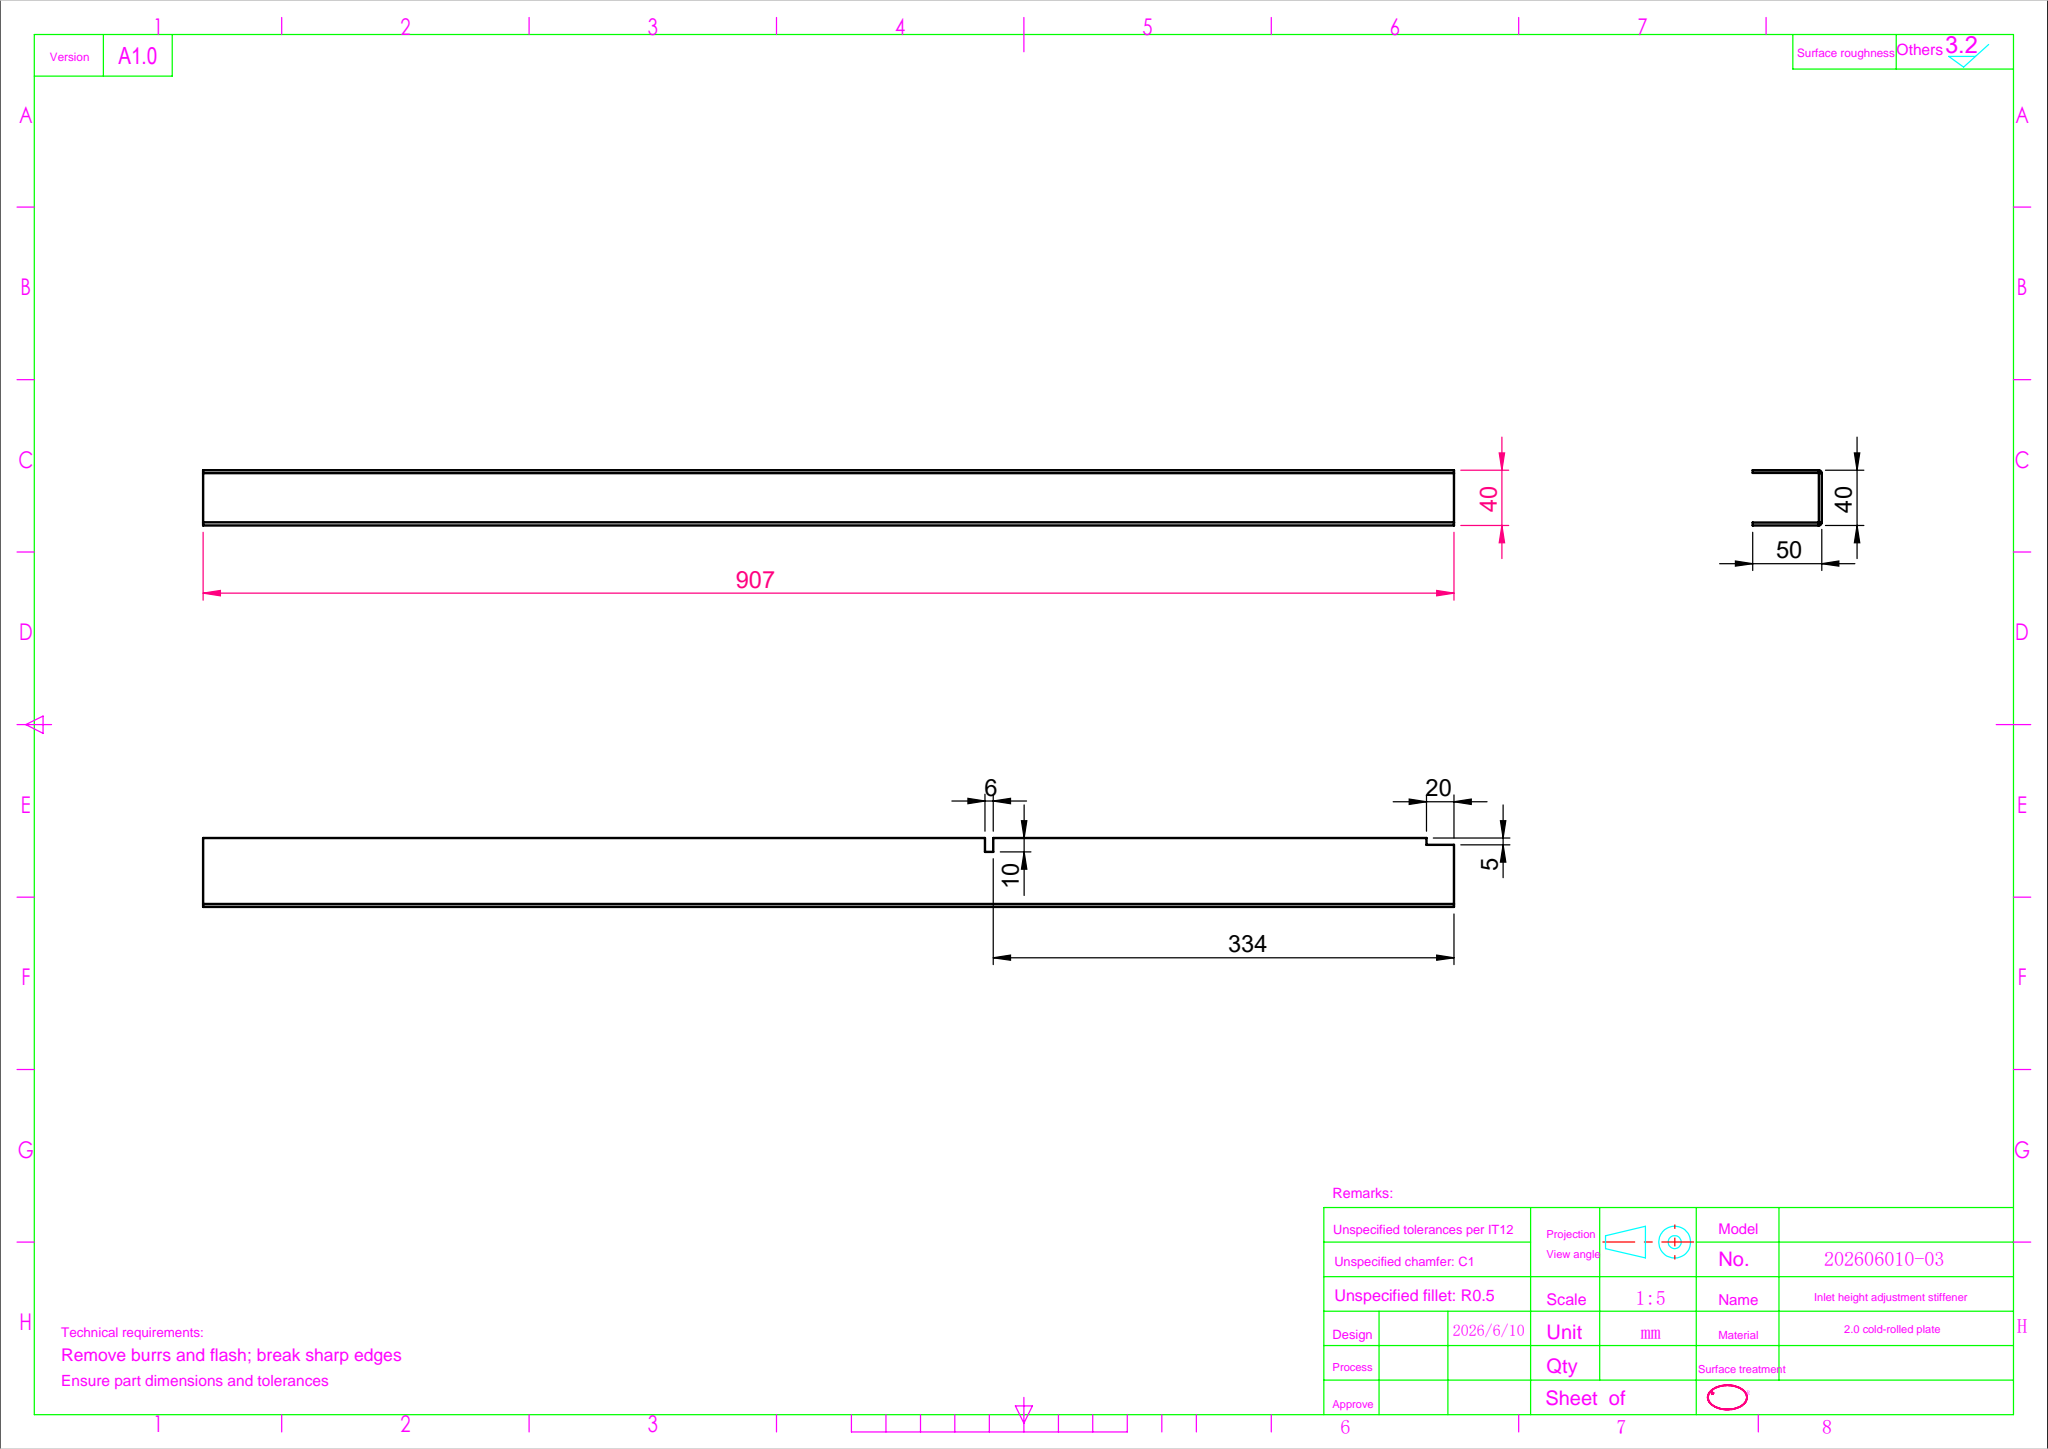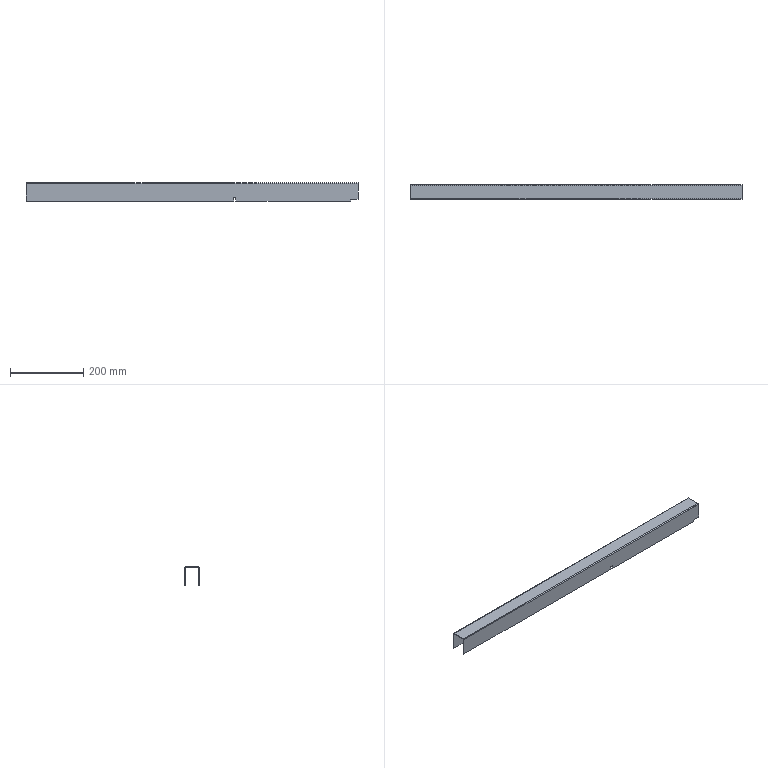Part | SolidWorks | features Cut 2, EdgeFlange 1, FlatPattern 1, SMBaseFlange 1, SheetMetal 1 | 1 solid | 34 faces | box 907 x 40 x 50 mm | volume 244195 mm3 | plane 30 | cylinder 4 | commonest cylinder face diameters 0.4 x2 4.4 x2
STEP:
#1=CARTESIAN_POINT('',(113.5,20.,-50.));
#2=VERTEX_POINT('',#1);
#3=CARTESIAN_POINT('',(-453.5,20.,-50.));
#4=VERTEX_POINT('',#3);
#5=CARTESIAN_POINT('',(0.,20.,-50.));
#6=DIRECTION('',(-1.,0.,0.));
#7=VECTOR('',#6,1000.);
#8=LINE('',#5,#7);
#9=EDGE_CURVE('',#2,#4,#8,.T.);
#10=ORIENTED_EDGE('',*,*,#9,.F.);
#11=CARTESIAN_POINT('',(113.5,18.,-50.));
#12=VERTEX_POINT('',#11);
#13=CARTESIAN_POINT('',(113.5,30.,-50.));
#14=DIRECTION('',(0.,-1.,0.));
#15=VECTOR('',#14,1000.);
#16=LINE('',#13,#15);
#17=EDGE_CURVE('',#2,#12,#16,.T.);
#18=ORIENTED_EDGE('',*,*,#17,.T.);
#19=CARTESIAN_POINT('',(-453.5,18.,-50.));
#20=VERTEX_POINT('',#19);
#21=CARTESIAN_POINT('',(-453.5,18.,-50.));
#22=DIRECTION('',(-1.,0.,0.));
#23=VECTOR('',#22,1000.);
#24=LINE('',#21,#23);
#25=EDGE_CURVE('',#12,#20,#24,.T.);
#26=ORIENTED_EDGE('',*,*,#25,.T.);
#27=CARTESIAN_POINT('',(-453.5,20.,-50.));
#28=DIRECTION('',(0.,-1.,0.));
#29=VECTOR('',#28,1000.);
#30=LINE('',#27,#29);
#31=EDGE_CURVE('',#4,#20,#30,.T.);
#32=ORIENTED_EDGE('',*,*,#31,.F.);
#33=EDGE_LOOP('',(#10,#18,#26,#32));
#34=FACE_OUTER_BOUND('',#33,.T.);
#35=CARTESIAN_POINT('',(-453.5,20.,-50.));
#36=DIRECTION('',(0.,0.,1.));
#37=DIRECTION('',(0.,-1.,0.));
#38=AXIS2_PLACEMENT_3D('',#35,#36,#37);
#39=PLANE('',#38);
#40=ADVANCED_FACE('',(#34),#39,.F.);
#41=CARTESIAN_POINT('',(-453.5,-18.,-50.));
#42=VERTEX_POINT('',#41);
#43=CARTESIAN_POINT('',(113.5,-18.,-50.));
#44=VERTEX_POINT('',#43);
#45=CARTESIAN_POINT('',(453.5,-18.,-50.));
#46=DIRECTION('',(1.,0.,0.));
#47=VECTOR('',#46,1000.);
#48=LINE('',#45,#47);
#49=EDGE_CURVE('',#42,#44,#48,.T.);
#50=ORIENTED_EDGE('',*,*,#49,.T.);
#51=CARTESIAN_POINT('',(113.5,-20.,-50.));
#52=VERTEX_POINT('',#51);
#53=CARTESIAN_POINT('',(113.5,-20.,-50.));
#54=DIRECTION('',(0.,-1.,0.));
#55=VECTOR('',#54,1000.);
#56=LINE('',#53,#55);
#57=EDGE_CURVE('',#44,#52,#56,.T.);
#58=ORIENTED_EDGE('',*,*,#57,.T.);
#59=CARTESIAN_POINT('',(-453.5,-20.,-50.));
#60=VERTEX_POINT('',#59);
#61=CARTESIAN_POINT('',(0.,-20.,-50.));
#62=DIRECTION('',(1.,0.,0.));
#63=VECTOR('',#62,1000.);
#64=LINE('',#61,#63);
#65=EDGE_CURVE('',#60,#52,#64,.T.);
#66=ORIENTED_EDGE('',*,*,#65,.F.);
#67=CARTESIAN_POINT('',(-453.5,-20.,-50.));
#68=DIRECTION('',(0.,1.,0.));
#69=VECTOR('',#68,1000.);
#70=LINE('',#67,#69);
#71=EDGE_CURVE('',#60,#42,#70,.T.);
#72=ORIENTED_EDGE('',*,*,#71,.T.);
#73=EDGE_LOOP('',(#50,#58,#66,#72));
#74=FACE_OUTER_BOUND('',#73,.T.);
#75=CARTESIAN_POINT('',(453.5,-20.,-50.));
#76=DIRECTION('',(0.,0.,1.));
#77=DIRECTION('',(0.,-1.,0.));
#78=AXIS2_PLACEMENT_3D('',#75,#76,#77);
#79=PLANE('',#78);
#80=ADVANCED_FACE('',(#74),#79,.F.);
#81=CARTESIAN_POINT('',(-453.5,-17.8,-2.));
#82=VERTEX_POINT('',#81);
#83=CARTESIAN_POINT('',(453.5,-17.8,-2.));
#84=VERTEX_POINT('',#83);
#85=CARTESIAN_POINT('',(-453.5,-17.8,-2.));
#86=DIRECTION('',(1.,0.,0.));
#87=VECTOR('',#86,1000.);
#88=LINE('',#85,#87);
#89=EDGE_CURVE('',#82,#84,#88,.T.);
#90=ORIENTED_EDGE('',*,*,#89,.F.);
#91=CARTESIAN_POINT('',(-453.5,17.8,-2.));
#92=VERTEX_POINT('',#91);
#93=CARTESIAN_POINT('',(-453.5,20.,-2.));
#94=DIRECTION('',(0.,-1.,0.));
#95=VECTOR('',#94,1000.);
#96=LINE('',#93,#95);
#97=EDGE_CURVE('',#92,#82,#96,.T.);
#98=ORIENTED_EDGE('',*,*,#97,.F.);
#99=CARTESIAN_POINT('',(453.5,17.8,-2.));
#100=VERTEX_POINT('',#99);
#101=CARTESIAN_POINT('',(453.5,17.8,-2.));
#102=DIRECTION('',(-1.,0.,0.));
#103=VECTOR('',#102,1000.);
#104=LINE('',#101,#103);
#105=EDGE_CURVE('',#100,#92,#104,.T.);
#106=ORIENTED_EDGE('',*,*,#105,.F.);
#107=CARTESIAN_POINT('',(453.5,20.,-2.));
#108=DIRECTION('',(0.,1.,0.));
#109=VECTOR('',#108,1000.);
#110=LINE('',#107,#109);
#111=EDGE_CURVE('',#84,#100,#110,.T.);
#112=ORIENTED_EDGE('',*,*,#111,.F.);
#113=EDGE_LOOP('',(#90,#98,#106,#112));
#114=FACE_OUTER_BOUND('',#113,.T.);
#115=CARTESIAN_POINT('',(0.,0.,-2.));
#116=DIRECTION('',(0.,0.,1.));
#117=DIRECTION('',(1.,0.,0.));
#118=AXIS2_PLACEMENT_3D('',#115,#116,#117);
#119=PLANE('',#118);
#120=ADVANCED_FACE('',(#114),#119,.F.);
#121=CARTESIAN_POINT('',(-453.5,17.8,0.));
#122=VERTEX_POINT('',#121);
#123=CARTESIAN_POINT('',(-453.5,-17.8,0.));
#124=VERTEX_POINT('',#123);
#125=CARTESIAN_POINT('',(-453.5,20.,0.));
#126=DIRECTION('',(0.,-1.,0.));
#127=VECTOR('',#126,1000.);
#128=LINE('',#125,#127);
#129=EDGE_CURVE('',#122,#124,#128,.T.);
#130=ORIENTED_EDGE('',*,*,#129,.T.);
#131=CARTESIAN_POINT('',(453.5,-17.8,0.));
#132=VERTEX_POINT('',#131);
#133=CARTESIAN_POINT('',(-453.5,-17.8,0.));
#134=DIRECTION('',(1.,0.,0.));
#135=VECTOR('',#134,1000.);
#136=LINE('',#133,#135);
#137=EDGE_CURVE('',#124,#132,#136,.T.);
#138=ORIENTED_EDGE('',*,*,#137,.T.);
#139=CARTESIAN_POINT('',(453.5,17.8,0.));
#140=VERTEX_POINT('',#139);
#141=CARTESIAN_POINT('',(453.5,20.,0.));
#142=DIRECTION('',(0.,1.,0.));
#143=VECTOR('',#142,1000.);
#144=LINE('',#141,#143);
#145=EDGE_CURVE('',#132,#140,#144,.T.);
#146=ORIENTED_EDGE('',*,*,#145,.T.);
#147=CARTESIAN_POINT('',(453.5,17.8,0.));
#148=DIRECTION('',(-1.,0.,0.));
#149=VECTOR('',#148,1000.);
#150=LINE('',#147,#149);
#151=EDGE_CURVE('',#140,#122,#150,.T.);
#152=ORIENTED_EDGE('',*,*,#151,.T.);
#153=EDGE_LOOP('',(#130,#138,#146,#152));
#154=FACE_OUTER_BOUND('',#153,.T.);
#155=CARTESIAN_POINT('',(0.,0.,0.));
#156=DIRECTION('',(0.,0.,1.));
#157=DIRECTION('',(1.,0.,0.));
#158=AXIS2_PLACEMENT_3D('',#155,#156,#157);
#159=PLANE('',#158);
#160=ADVANCED_FACE('',(#154),#159,.T.);
#161=ORIENTED_EDGE('',*,*,#97,.T.);
#162=CARTESIAN_POINT('',(-453.5,-17.8,-2.));
#163=DIRECTION('',(0.,0.,1.));
#164=VECTOR('',#163,1000.);
#165=LINE('',#162,#164);
#166=EDGE_CURVE('',#82,#124,#165,.T.);
#167=ORIENTED_EDGE('',*,*,#166,.T.);
#168=ORIENTED_EDGE('',*,*,#129,.F.);
#169=CARTESIAN_POINT('',(-453.5,17.8,-2.));
#170=DIRECTION('',(0.,0.,1.));
#171=VECTOR('',#170,1000.);
#172=LINE('',#169,#171);
#173=EDGE_CURVE('',#92,#122,#172,.T.);
#174=ORIENTED_EDGE('',*,*,#173,.F.);
#175=EDGE_LOOP('',(#161,#167,#168,#174));
#176=FACE_OUTER_BOUND('',#175,.T.);
#177=CARTESIAN_POINT('',(-453.5,20.,-2.));
#178=DIRECTION('',(-1.,0.,0.));
#179=DIRECTION('',(0.,0.,1.));
#180=AXIS2_PLACEMENT_3D('',#177,#178,#179);
#181=PLANE('',#180);
#182=ADVANCED_FACE('',(#176),#181,.T.);
#183=CARTESIAN_POINT('',(453.5,-17.8,-2.));
#184=DIRECTION('',(0.,0.,1.));
#185=VECTOR('',#184,1000.);
#186=LINE('',#183,#185);
#187=EDGE_CURVE('',#84,#132,#186,.T.);
#188=ORIENTED_EDGE('',*,*,#187,.F.);
#189=ORIENTED_EDGE('',*,*,#111,.T.);
#190=CARTESIAN_POINT('',(453.5,17.8,-2.));
#191=DIRECTION('',(0.,0.,1.));
#192=VECTOR('',#191,1000.);
#193=LINE('',#190,#192);
#194=EDGE_CURVE('',#100,#140,#193,.T.);
#195=ORIENTED_EDGE('',*,*,#194,.T.);
#196=ORIENTED_EDGE('',*,*,#145,.F.);
#197=EDGE_LOOP('',(#188,#189,#195,#196));
#198=FACE_OUTER_BOUND('',#197,.T.);
#199=CARTESIAN_POINT('',(453.5,20.,-2.));
#200=DIRECTION('',(1.,0.,0.));
#201=DIRECTION('',(0.,0.,-1.));
#202=AXIS2_PLACEMENT_3D('',#199,#200,#201);
#203=PLANE('',#202);
#204=ADVANCED_FACE('',(#198),#203,.T.);
#205=CARTESIAN_POINT('',(-453.5,18.,-2.2));
#206=VERTEX_POINT('',#205);
#207=CARTESIAN_POINT('',(-453.5,20.,-2.2));
#208=VERTEX_POINT('',#207);
#209=CARTESIAN_POINT('',(-453.5,20.,-2.2));
#210=DIRECTION('',(0.,1.,0.));
#211=VECTOR('',#210,1000.);
#212=LINE('',#209,#211);
#213=EDGE_CURVE('',#206,#208,#212,.T.);
#214=ORIENTED_EDGE('',*,*,#213,.F.);
#215=CARTESIAN_POINT('',(-453.5,17.8,-2.2));
#216=DIRECTION('',(-1.,0.,0.));
#217=DIRECTION('',(0.,0.,-1.));
#218=AXIS2_PLACEMENT_3D('',#215,#216,#217);
#219=CIRCLE('',#218,0.2);
#220=EDGE_CURVE('',#92,#206,#219,.T.);
#221=ORIENTED_EDGE('',*,*,#220,.F.);
#222=ORIENTED_EDGE('',*,*,#173,.T.);
#223=CARTESIAN_POINT('',(-453.5,17.8,-2.2));
#224=DIRECTION('',(-1.,0.,0.));
#225=DIRECTION('',(0.,0.,-1.));
#226=AXIS2_PLACEMENT_3D('',#223,#224,#225);
#227=CIRCLE('',#226,2.2);
#228=EDGE_CURVE('',#122,#208,#227,.T.);
#229=ORIENTED_EDGE('',*,*,#228,.T.);
#230=EDGE_LOOP('',(#214,#221,#222,#229));
#231=FACE_OUTER_BOUND('',#230,.T.);
#232=CARTESIAN_POINT('',(-453.5,17.8,-2.2));
#233=DIRECTION('',(-1.,0.,0.));
#234=DIRECTION('',(0.,0.,1.));
#235=AXIS2_PLACEMENT_3D('',#232,#233,#234);
#236=PLANE('',#235);
#237=ADVANCED_FACE('',(#231),#236,.T.);
#238=CARTESIAN_POINT('',(453.5,18.,-2.2));
#239=VERTEX_POINT('',#238);
#240=CARTESIAN_POINT('',(453.5,17.8,-2.2));
#241=DIRECTION('',(1.,0.,0.));
#242=DIRECTION('',(0.,0.,-1.));
#243=AXIS2_PLACEMENT_3D('',#240,#241,#242);
#244=CIRCLE('',#243,0.2);
#245=EDGE_CURVE('',#239,#100,#244,.T.);
#246=ORIENTED_EDGE('',*,*,#245,.F.);
#247=CARTESIAN_POINT('',(453.5,20.,-2.2));
#248=VERTEX_POINT('',#247);
#249=CARTESIAN_POINT('',(453.5,18.,-2.2));
#250=DIRECTION('',(0.,1.,0.));
#251=VECTOR('',#250,1000.);
#252=LINE('',#249,#251);
#253=EDGE_CURVE('',#239,#248,#252,.T.);
#254=ORIENTED_EDGE('',*,*,#253,.T.);
#255=CARTESIAN_POINT('',(453.5,17.8,-2.2));
#256=DIRECTION('',(1.,0.,0.));
#257=DIRECTION('',(0.,0.,-1.));
#258=AXIS2_PLACEMENT_3D('',#255,#256,#257);
#259=CIRCLE('',#258,2.2);
#260=EDGE_CURVE('',#248,#140,#259,.T.);
#261=ORIENTED_EDGE('',*,*,#260,.T.);
#262=ORIENTED_EDGE('',*,*,#194,.F.);
#263=EDGE_LOOP('',(#246,#254,#261,#262));
#264=FACE_OUTER_BOUND('',#263,.T.);
#265=CARTESIAN_POINT('',(453.5,17.8,-2.2));
#266=DIRECTION('',(-1.,0.,0.));
#267=DIRECTION('',(0.,0.,1.));
#268=AXIS2_PLACEMENT_3D('',#265,#266,#267);
#269=PLANE('',#268);
#270=ADVANCED_FACE('',(#264),#269,.F.);
#271=ORIENTED_EDGE('',*,*,#151,.F.);
#272=ORIENTED_EDGE('',*,*,#260,.F.);
#273=CARTESIAN_POINT('',(-453.5,20.,-2.2));
#274=DIRECTION('',(-1.,0.,0.));
#275=VECTOR('',#274,1000.);
#276=LINE('',#273,#275);
#277=EDGE_CURVE('',#248,#208,#276,.T.);
#278=ORIENTED_EDGE('',*,*,#277,.T.);
#279=ORIENTED_EDGE('',*,*,#228,.F.);
#280=EDGE_LOOP('',(#271,#272,#278,#279));
#281=FACE_OUTER_BOUND('',#280,.T.);
#282=CARTESIAN_POINT('',(453.5,17.8,-2.2));
#283=DIRECTION('',(1.,0.,0.));
#284=DIRECTION('',(0.,1.,0.));
#285=AXIS2_PLACEMENT_3D('',#282,#283,#284);
#286=CYLINDRICAL_SURFACE('',#285,2.2);
#287=ADVANCED_FACE('',(#281),#286,.T.);
#288=ORIENTED_EDGE('',*,*,#105,.T.);
#289=ORIENTED_EDGE('',*,*,#220,.T.);
#290=CARTESIAN_POINT('',(-453.5,18.,-2.2));
#291=DIRECTION('',(1.,0.,0.));
#292=VECTOR('',#291,1000.);
#293=LINE('',#290,#292);
#294=EDGE_CURVE('',#206,#239,#293,.T.);
#295=ORIENTED_EDGE('',*,*,#294,.T.);
#296=ORIENTED_EDGE('',*,*,#245,.T.);
#297=EDGE_LOOP('',(#288,#289,#295,#296));
#298=FACE_OUTER_BOUND('',#297,.T.);
#299=CARTESIAN_POINT('',(453.5,17.8,-2.2));
#300=DIRECTION('',(1.,0.,0.));
#301=DIRECTION('',(0.,1.,0.));
#302=AXIS2_PLACEMENT_3D('',#299,#300,#301);
#303=CYLINDRICAL_SURFACE('',#302,0.2);
#304=ADVANCED_FACE('',(#298),#303,.F.);
#305=CARTESIAN_POINT('',(453.5,18.,-45.));
#306=VERTEX_POINT('',#305);
#307=CARTESIAN_POINT('',(453.5,18.,-50.));
#308=DIRECTION('',(0.,0.,-1.));
#309=VECTOR('',#308,1000.);
#310=LINE('',#307,#309);
#311=EDGE_CURVE('',#239,#306,#310,.T.);
#312=ORIENTED_EDGE('',*,*,#311,.T.);
#313=CARTESIAN_POINT('',(453.5,20.,-45.));
#314=VERTEX_POINT('',#313);
#315=CARTESIAN_POINT('',(453.5,30.,-45.));
#316=DIRECTION('',(0.,-1.,0.));
#317=VECTOR('',#316,1000.);
#318=LINE('',#315,#317);
#319=EDGE_CURVE('',#314,#306,#318,.T.);
#320=ORIENTED_EDGE('',*,*,#319,.F.);
#321=CARTESIAN_POINT('',(453.5,20.,0.));
#322=DIRECTION('',(0.,0.,-1.));
#323=VECTOR('',#322,1000.);
#324=LINE('',#321,#323);
#325=EDGE_CURVE('',#248,#314,#324,.T.);
#326=ORIENTED_EDGE('',*,*,#325,.F.);
#327=ORIENTED_EDGE('',*,*,#253,.F.);
#328=EDGE_LOOP('',(#312,#320,#326,#327));
#329=FACE_OUTER_BOUND('',#328,.T.);
#330=CARTESIAN_POINT('',(453.5,20.,-50.));
#331=DIRECTION('',(-1.,0.,0.));
#332=DIRECTION('',(0.,0.,1.));
#333=AXIS2_PLACEMENT_3D('',#330,#331,#332);
#334=PLANE('',#333);
#335=ADVANCED_FACE('',(#329),#334,.F.);
#336=ORIENTED_EDGE('',*,*,#213,.T.);
#337=CARTESIAN_POINT('',(-453.5,20.,0.));
#338=DIRECTION('',(0.,0.,1.));
#339=VECTOR('',#338,1000.);
#340=LINE('',#337,#339);
#341=EDGE_CURVE('',#4,#208,#340,.T.);
#342=ORIENTED_EDGE('',*,*,#341,.F.);
#343=ORIENTED_EDGE('',*,*,#31,.T.);
#344=CARTESIAN_POINT('',(-453.5,18.,-2.));
#345=DIRECTION('',(0.,0.,1.));
#346=VECTOR('',#345,1000.);
#347=LINE('',#344,#346);
#348=EDGE_CURVE('',#20,#206,#347,.T.);
#349=ORIENTED_EDGE('',*,*,#348,.T.);
#350=EDGE_LOOP('',(#336,#342,#343,#349));
#351=FACE_OUTER_BOUND('',#350,.T.);
#352=CARTESIAN_POINT('',(-453.5,20.,-2.));
#353=DIRECTION('',(1.,0.,0.));
#354=DIRECTION('',(0.,0.,-1.));
#355=AXIS2_PLACEMENT_3D('',#352,#353,#354);
#356=PLANE('',#355);
#357=ADVANCED_FACE('',(#351),#356,.F.);
#358=CARTESIAN_POINT('',(433.5,20.,-45.));
#359=VERTEX_POINT('',#358);
#360=CARTESIAN_POINT('',(0.,20.,-45.));
#361=DIRECTION('',(-1.,0.,0.));
#362=VECTOR('',#361,1000.);
#363=LINE('',#360,#362);
#364=EDGE_CURVE('',#314,#359,#363,.T.);
#365=ORIENTED_EDGE('',*,*,#364,.T.);
#366=CARTESIAN_POINT('',(433.5,20.,-50.));
#367=VERTEX_POINT('',#366);
#368=CARTESIAN_POINT('',(433.5,20.,0.));
#369=DIRECTION('',(0.,0.,-1.));
#370=VECTOR('',#369,1000.);
#371=LINE('',#368,#370);
#372=EDGE_CURVE('',#359,#367,#371,.T.);
#373=ORIENTED_EDGE('',*,*,#372,.T.);
#374=CARTESIAN_POINT('',(119.5,20.,-50.));
#375=VERTEX_POINT('',#374);
#376=CARTESIAN_POINT('',(0.,20.,-50.));
#377=DIRECTION('',(-1.,0.,0.));
#378=VECTOR('',#377,1000.);
#379=LINE('',#376,#378);
#380=EDGE_CURVE('',#367,#375,#379,.T.);
#381=ORIENTED_EDGE('',*,*,#380,.T.);
#382=CARTESIAN_POINT('',(119.5,20.,-40.));
#383=VERTEX_POINT('',#382);
#384=CARTESIAN_POINT('',(119.5,20.,0.));
#385=DIRECTION('',(0.,0.,1.));
#386=VECTOR('',#385,1000.);
#387=LINE('',#384,#386);
#388=EDGE_CURVE('',#375,#383,#387,.T.);
#389=ORIENTED_EDGE('',*,*,#388,.T.);
#390=CARTESIAN_POINT('',(113.5,20.,-40.));
#391=VERTEX_POINT('',#390);
#392=CARTESIAN_POINT('',(0.,20.,-40.));
#393=DIRECTION('',(-1.,0.,0.));
#394=VECTOR('',#393,1000.);
#395=LINE('',#392,#394);
#396=EDGE_CURVE('',#383,#391,#395,.T.);
#397=ORIENTED_EDGE('',*,*,#396,.T.);
#398=CARTESIAN_POINT('',(113.5,20.,0.));
#399=DIRECTION('',(0.,0.,-1.));
#400=VECTOR('',#399,1000.);
#401=LINE('',#398,#400);
#402=EDGE_CURVE('',#391,#2,#401,.T.);
#403=ORIENTED_EDGE('',*,*,#402,.T.);
#404=ORIENTED_EDGE('',*,*,#9,.T.);
#405=ORIENTED_EDGE('',*,*,#341,.T.);
#406=ORIENTED_EDGE('',*,*,#277,.F.);
#407=ORIENTED_EDGE('',*,*,#325,.T.);
#408=EDGE_LOOP('',(#365,#373,#381,#389,#397,#403,#404,#405,#406,#407));
#409=FACE_OUTER_BOUND('',#408,.T.);
#410=CARTESIAN_POINT('',(0.,20.,0.));
#411=DIRECTION('',(0.,-1.,0.));
#412=DIRECTION('',(0.,0.,-1.));
#413=AXIS2_PLACEMENT_3D('',#410,#411,#412);
#414=PLANE('',#413);
#415=ADVANCED_FACE('',(#409),#414,.F.);
#416=CARTESIAN_POINT('',(433.5,18.,-45.));
#417=VERTEX_POINT('',#416);
#418=CARTESIAN_POINT('',(433.5,18.,-50.));
#419=VERTEX_POINT('',#418);
#420=CARTESIAN_POINT('',(433.5,18.,0.));
#421=DIRECTION('',(0.,0.,-1.));
#422=VECTOR('',#421,1000.);
#423=LINE('',#420,#422);
#424=EDGE_CURVE('',#417,#419,#423,.T.);
#425=ORIENTED_EDGE('',*,*,#424,.F.);
#426=CARTESIAN_POINT('',(0.,18.,-45.));
#427=DIRECTION('',(-1.,0.,0.));
#428=VECTOR('',#427,1000.);
#429=LINE('',#426,#428);
#430=EDGE_CURVE('',#306,#417,#429,.T.);
#431=ORIENTED_EDGE('',*,*,#430,.F.);
#432=ORIENTED_EDGE('',*,*,#311,.F.);
#433=ORIENTED_EDGE('',*,*,#294,.F.);
#434=ORIENTED_EDGE('',*,*,#348,.F.);
#435=ORIENTED_EDGE('',*,*,#25,.F.);
#436=CARTESIAN_POINT('',(113.5,18.,-40.));
#437=VERTEX_POINT('',#436);
#438=CARTESIAN_POINT('',(113.5,18.,0.));
#439=DIRECTION('',(0.,0.,-1.));
#440=VECTOR('',#439,1000.);
#441=LINE('',#438,#440);
#442=EDGE_CURVE('',#437,#12,#441,.T.);
#443=ORIENTED_EDGE('',*,*,#442,.F.);
#444=CARTESIAN_POINT('',(119.5,18.,-40.));
#445=VERTEX_POINT('',#444);
#446=CARTESIAN_POINT('',(0.,18.,-40.));
#447=DIRECTION('',(-1.,0.,0.));
#448=VECTOR('',#447,1000.);
#449=LINE('',#446,#448);
#450=EDGE_CURVE('',#445,#437,#449,.T.);
#451=ORIENTED_EDGE('',*,*,#450,.F.);
#452=CARTESIAN_POINT('',(119.5,18.,-50.));
#453=VERTEX_POINT('',#452);
#454=CARTESIAN_POINT('',(119.5,18.,0.));
#455=DIRECTION('',(0.,0.,1.));
#456=VECTOR('',#455,1000.);
#457=LINE('',#454,#456);
#458=EDGE_CURVE('',#453,#445,#457,.T.);
#459=ORIENTED_EDGE('',*,*,#458,.F.);
#460=CARTESIAN_POINT('',(-453.5,18.,-50.));
#461=DIRECTION('',(-1.,0.,0.));
#462=VECTOR('',#461,1000.);
#463=LINE('',#460,#462);
#464=EDGE_CURVE('',#419,#453,#463,.T.);
#465=ORIENTED_EDGE('',*,*,#464,.F.);
#466=EDGE_LOOP('',(#425,#431,#432,#433,#434,#435,#443,#451,#459,#465));
#467=FACE_OUTER_BOUND('',#466,.T.);
#468=CARTESIAN_POINT('',(0.,18.,0.));
#469=DIRECTION('',(0.,-1.,0.));
#470=DIRECTION('',(0.,0.,-1.));
#471=AXIS2_PLACEMENT_3D('',#468,#469,#470);
#472=PLANE('',#471);
#473=ADVANCED_FACE('',(#467),#472,.T.);
#474=ORIENTED_EDGE('',*,*,#380,.F.);
#475=CARTESIAN_POINT('',(433.5,30.,-50.));
#476=DIRECTION('',(0.,-1.,0.));
#477=VECTOR('',#476,1000.);
#478=LINE('',#475,#477);
#479=EDGE_CURVE('',#367,#419,#478,.T.);
#480=ORIENTED_EDGE('',*,*,#479,.T.);
#481=ORIENTED_EDGE('',*,*,#464,.T.);
#482=CARTESIAN_POINT('',(119.5,30.,-50.));
#483=DIRECTION('',(0.,-1.,0.));
#484=VECTOR('',#483,1000.);
#485=LINE('',#482,#484);
#486=EDGE_CURVE('',#375,#453,#485,.T.);
#487=ORIENTED_EDGE('',*,*,#486,.F.);
#488=EDGE_LOOP('',(#474,#480,#481,#487));
#489=FACE_OUTER_BOUND('',#488,.T.);
#490=CARTESIAN_POINT('',(-453.5,20.,-50.));
#491=DIRECTION('',(0.,0.,1.));
#492=DIRECTION('',(0.,-1.,0.));
#493=AXIS2_PLACEMENT_3D('',#490,#491,#492);
#494=PLANE('',#493);
#495=ADVANCED_FACE('',(#489),#494,.F.);
#496=CARTESIAN_POINT('',(453.5,-18.,-2.2));
#497=VERTEX_POINT('',#496);
#498=CARTESIAN_POINT('',(453.5,-20.,-2.2));
#499=VERTEX_POINT('',#498);
#500=CARTESIAN_POINT('',(453.5,-20.,-2.2));
#501=DIRECTION('',(0.,-1.,0.));
#502=VECTOR('',#501,1000.);
#503=LINE('',#500,#502);
#504=EDGE_CURVE('',#497,#499,#503,.T.);
#505=ORIENTED_EDGE('',*,*,#504,.F.);
#506=CARTESIAN_POINT('',(453.5,-17.8,-2.2));
#507=DIRECTION('',(1.,0.,0.));
#508=DIRECTION('',(0.,0.,1.));
#509=AXIS2_PLACEMENT_3D('',#506,#507,#508);
#510=CIRCLE('',#509,0.2);
#511=EDGE_CURVE('',#84,#497,#510,.T.);
#512=ORIENTED_EDGE('',*,*,#511,.F.);
#513=ORIENTED_EDGE('',*,*,#187,.T.);
#514=CARTESIAN_POINT('',(453.5,-17.8,-2.2));
#515=DIRECTION('',(1.,0.,0.));
#516=DIRECTION('',(0.,0.,1.));
#517=AXIS2_PLACEMENT_3D('',#514,#515,#516);
#518=CIRCLE('',#517,2.2);
#519=EDGE_CURVE('',#132,#499,#518,.T.);
#520=ORIENTED_EDGE('',*,*,#519,.T.);
#521=EDGE_LOOP('',(#505,#512,#513,#520));
#522=FACE_OUTER_BOUND('',#521,.T.);
#523=CARTESIAN_POINT('',(453.5,-17.8,-2.2));
#524=DIRECTION('',(1.,0.,0.));
#525=DIRECTION('',(0.,0.,-1.));
#526=AXIS2_PLACEMENT_3D('',#523,#524,#525);
#527=PLANE('',#526);
#528=ADVANCED_FACE('',(#522),#527,.T.);
#529=CARTESIAN_POINT('',(-453.5,-18.,-2.2));
#530=VERTEX_POINT('',#529);
#531=CARTESIAN_POINT('',(-453.5,-17.8,-2.2));
#532=DIRECTION('',(-1.,0.,0.));
#533=DIRECTION('',(0.,0.,1.));
#534=AXIS2_PLACEMENT_3D('',#531,#532,#533);
#535=CIRCLE('',#534,0.2);
#536=EDGE_CURVE('',#530,#82,#535,.T.);
#537=ORIENTED_EDGE('',*,*,#536,.F.);
#538=CARTESIAN_POINT('',(-453.5,-20.,-2.2));
#539=VERTEX_POINT('',#538);
#540=CARTESIAN_POINT('',(-453.5,-18.,-2.2));
#541=DIRECTION('',(0.,-1.,0.));
#542=VECTOR('',#541,1000.);
#543=LINE('',#540,#542);
#544=EDGE_CURVE('',#530,#539,#543,.T.);
#545=ORIENTED_EDGE('',*,*,#544,.T.);
#546=CARTESIAN_POINT('',(-453.5,-17.8,-2.2));
#547=DIRECTION('',(-1.,0.,0.));
#548=DIRECTION('',(0.,0.,1.));
#549=AXIS2_PLACEMENT_3D('',#546,#547,#548);
#550=CIRCLE('',#549,2.2);
#551=EDGE_CURVE('',#539,#124,#550,.T.);
#552=ORIENTED_EDGE('',*,*,#551,.T.);
#553=ORIENTED_EDGE('',*,*,#166,.F.);
#554=EDGE_LOOP('',(#537,#545,#552,#553));
#555=FACE_OUTER_BOUND('',#554,.T.);
#556=CARTESIAN_POINT('',(-453.5,-17.8,-2.2));
#557=DIRECTION('',(1.,0.,0.));
#558=DIRECTION('',(0.,0.,-1.));
#559=AXIS2_PLACEMENT_3D('',#556,#557,#558);
#560=PLANE('',#559);
#561=ADVANCED_FACE('',(#555),#560,.F.);
#562=ORIENTED_EDGE('',*,*,#137,.F.);
#563=ORIENTED_EDGE('',*,*,#551,.F.);
#564=CARTESIAN_POINT('',(453.5,-20.,-2.2));
#565=DIRECTION('',(1.,0.,0.));
#566=VECTOR('',#565,1000.);
#567=LINE('',#564,#566);
#568=EDGE_CURVE('',#539,#499,#567,.T.);
#569=ORIENTED_EDGE('',*,*,#568,.T.);
#570=ORIENTED_EDGE('',*,*,#519,.F.);
#571=EDGE_LOOP('',(#562,#563,#569,#570));
#572=FACE_OUTER_BOUND('',#571,.T.);
#573=CARTESIAN_POINT('',(-453.5,-17.8,-2.2));
#574=DIRECTION('',(-1.,0.,0.));
#575=DIRECTION('',(0.,-1.,0.));
#576=AXIS2_PLACEMENT_3D('',#573,#574,#575);
#577=CYLINDRICAL_SURFACE('',#576,2.2);
#578=ADVANCED_FACE('',(#572),#577,.T.);
#579=ORIENTED_EDGE('',*,*,#89,.T.);
#580=ORIENTED_EDGE('',*,*,#511,.T.);
#581=CARTESIAN_POINT('',(453.5,-18.,-2.2));
#582=DIRECTION('',(-1.,0.,0.));
#583=VECTOR('',#582,1000.);
#584=LINE('',#581,#583);
#585=EDGE_CURVE('',#497,#530,#584,.T.);
#586=ORIENTED_EDGE('',*,*,#585,.T.);
#587=ORIENTED_EDGE('',*,*,#536,.T.);
#588=EDGE_LOOP('',(#579,#580,#586,#587));
#589=FACE_OUTER_BOUND('',#588,.T.);
#590=CARTESIAN_POINT('',(-453.5,-17.8,-2.2));
#591=DIRECTION('',(-1.,0.,0.));
#592=DIRECTION('',(0.,-1.,0.));
#593=AXIS2_PLACEMENT_3D('',#590,#591,#592);
#594=CYLINDRICAL_SURFACE('',#593,0.2);
#595=ADVANCED_FACE('',(#589),#594,.F.);
#596=ORIENTED_EDGE('',*,*,#544,.F.);
#597=CARTESIAN_POINT('',(-453.5,-18.,-50.));
#598=DIRECTION('',(0.,0.,-1.));
#599=VECTOR('',#598,1000.);
#600=LINE('',#597,#599);
#601=EDGE_CURVE('',#530,#42,#600,.T.);
#602=ORIENTED_EDGE('',*,*,#601,.T.);
#603=ORIENTED_EDGE('',*,*,#71,.F.);
#604=CARTESIAN_POINT('',(-453.5,-20.,0.));
#605=DIRECTION('',(0.,0.,-1.));
#606=VECTOR('',#605,1000.);
#607=LINE('',#604,#606);
#608=EDGE_CURVE('',#539,#60,#607,.T.);
#609=ORIENTED_EDGE('',*,*,#608,.F.);
#610=EDGE_LOOP('',(#596,#602,#603,#609));
#611=FACE_OUTER_BOUND('',#610,.T.);
#612=CARTESIAN_POINT('',(-453.5,-20.,-50.));
#613=DIRECTION('',(1.,0.,0.));
#614=DIRECTION('',(0.,0.,-1.));
#615=AXIS2_PLACEMENT_3D('',#612,#613,#614);
#616=PLANE('',#615);
#617=ADVANCED_FACE('',(#611),#616,.F.);
#618=CARTESIAN_POINT('',(453.5,-20.,-45.));
#619=VERTEX_POINT('',#618);
#620=CARTESIAN_POINT('',(453.5,-20.,0.));
#621=DIRECTION('',(0.,0.,1.));
#622=VECTOR('',#621,1000.);
#623=LINE('',#620,#622);
#624=EDGE_CURVE('',#619,#499,#623,.T.);
#625=ORIENTED_EDGE('',*,*,#624,.F.);
#626=CARTESIAN_POINT('',(453.5,-18.,-45.));
#627=VERTEX_POINT('',#626);
#628=CARTESIAN_POINT('',(453.5,30.,-45.));
#629=DIRECTION('',(0.,-1.,0.));
#630=VECTOR('',#629,1000.);
#631=LINE('',#628,#630);
#632=EDGE_CURVE('',#627,#619,#631,.T.);
#633=ORIENTED_EDGE('',*,*,#632,.F.);
#634=CARTESIAN_POINT('',(453.5,-18.,-2.));
#635=DIRECTION('',(0.,0.,1.));
#636=VECTOR('',#635,1000.);
#637=LINE('',#634,#636);
#638=EDGE_CURVE('',#627,#497,#637,.T.);
#639=ORIENTED_EDGE('',*,*,#638,.T.);
#640=ORIENTED_EDGE('',*,*,#504,.T.);
#641=EDGE_LOOP('',(#625,#633,#639,#640));
#642=FACE_OUTER_BOUND('',#641,.T.);
#643=CARTESIAN_POINT('',(453.5,-20.,-2.));
#644=DIRECTION('',(-1.,0.,0.));
#645=DIRECTION('',(0.,0.,1.));
#646=AXIS2_PLACEMENT_3D('',#643,#644,#645);
#647=PLANE('',#646);
#648=ADVANCED_FACE('',(#642),#647,.F.);
#649=CARTESIAN_POINT('',(119.5,-20.,-50.));
#650=VERTEX_POINT('',#649);
#651=CARTESIAN_POINT('',(433.5,-20.,-50.));
#652=VERTEX_POINT('',#651);
#653=CARTESIAN_POINT('',(0.,-20.,-50.));
#654=DIRECTION('',(1.,0.,0.));
#655=VECTOR('',#654,1000.);
#656=LINE('',#653,#655);
#657=EDGE_CURVE('',#650,#652,#656,.T.);
#658=ORIENTED_EDGE('',*,*,#657,.T.);
#659=CARTESIAN_POINT('',(433.5,-20.,-45.));
#660=VERTEX_POINT('',#659);
#661=CARTESIAN_POINT('',(433.5,-20.,-50.));
#662=DIRECTION('',(0.,0.,-1.));
#663=VECTOR('',#662,1000.);
#664=LINE('',#661,#663);
#665=EDGE_CURVE('',#660,#652,#664,.T.);
#666=ORIENTED_EDGE('',*,*,#665,.F.);
#667=CARTESIAN_POINT('',(433.5,-20.,-45.));
#668=DIRECTION('',(-1.,0.,0.));
#669=VECTOR('',#668,1000.);
#670=LINE('',#667,#669);
#671=EDGE_CURVE('',#619,#660,#670,.T.);
#672=ORIENTED_EDGE('',*,*,#671,.F.);
#673=ORIENTED_EDGE('',*,*,#624,.T.);
#674=ORIENTED_EDGE('',*,*,#568,.F.);
#675=ORIENTED_EDGE('',*,*,#608,.T.);
#676=ORIENTED_EDGE('',*,*,#65,.T.);
#677=CARTESIAN_POINT('',(113.5,-20.,-40.));
#678=VERTEX_POINT('',#677);
#679=CARTESIAN_POINT('',(113.5,-20.,-50.));
#680=DIRECTION('',(0.,0.,-1.));
#681=VECTOR('',#680,1000.);
#682=LINE('',#679,#681);
#683=EDGE_CURVE('',#678,#52,#682,.T.);
#684=ORIENTED_EDGE('',*,*,#683,.F.);
#685=CARTESIAN_POINT('',(119.5,-20.,-40.));
#686=VERTEX_POINT('',#685);
#687=CARTESIAN_POINT('',(113.5,-20.,-40.));
#688=DIRECTION('',(-1.,0.,0.));
#689=VECTOR('',#688,1000.);
#690=LINE('',#687,#689);
#691=EDGE_CURVE('',#686,#678,#690,.T.);
#692=ORIENTED_EDGE('',*,*,#691,.F.);
#693=CARTESIAN_POINT('',(119.5,-20.,-50.));
#694=DIRECTION('',(0.,0.,1.));
#695=VECTOR('',#694,1000.);
#696=LINE('',#693,#695);
#697=EDGE_CURVE('',#650,#686,#696,.T.);
#698=ORIENTED_EDGE('',*,*,#697,.F.);
#699=EDGE_LOOP('',(#658,#666,#672,#673,#674,#675,#676,#684,#692,#698));
#700=FACE_OUTER_BOUND('',#699,.T.);
#701=CARTESIAN_POINT('',(0.,-20.,0.));
#702=DIRECTION('',(0.,1.,0.));
#703=DIRECTION('',(0.,0.,1.));
#704=AXIS2_PLACEMENT_3D('',#701,#702,#703);
#705=PLANE('',#704);
#706=ADVANCED_FACE('',(#700),#705,.F.);
#707=CARTESIAN_POINT('',(433.5,-18.,-50.));
#708=VERTEX_POINT('',#707);
#709=CARTESIAN_POINT('',(433.5,-18.,-45.));
#710=VERTEX_POINT('',#709);
#711=CARTESIAN_POINT('',(433.5,-18.,0.));
#712=DIRECTION('',(0.,0.,1.));
#713=VECTOR('',#712,1000.);
#714=LINE('',#711,#713);
#715=EDGE_CURVE('',#708,#710,#714,.T.);
#716=ORIENTED_EDGE('',*,*,#715,.F.);
#717=CARTESIAN_POINT('',(119.5,-18.,-50.));
#718=VERTEX_POINT('',#717);
#719=CARTESIAN_POINT('',(453.5,-18.,-50.));
#720=DIRECTION('',(1.,0.,0.));
#721=VECTOR('',#720,1000.);
#722=LINE('',#719,#721);
#723=EDGE_CURVE('',#718,#708,#722,.T.);
#724=ORIENTED_EDGE('',*,*,#723,.F.);
#725=CARTESIAN_POINT('',(119.5,-18.,-40.));
#726=VERTEX_POINT('',#725);
#727=CARTESIAN_POINT('',(119.5,-18.,0.));
#728=DIRECTION('',(0.,0.,-1.));
#729=VECTOR('',#728,1000.);
#730=LINE('',#727,#729);
#731=EDGE_CURVE('',#726,#718,#730,.T.);
#732=ORIENTED_EDGE('',*,*,#731,.F.);
#733=CARTESIAN_POINT('',(113.5,-18.,-40.));
#734=VERTEX_POINT('',#733);
#735=CARTESIAN_POINT('',(0.,-18.,-40.));
#736=DIRECTION('',(1.,0.,0.));
#737=VECTOR('',#736,1000.);
#738=LINE('',#735,#737);
#739=EDGE_CURVE('',#734,#726,#738,.T.);
#740=ORIENTED_EDGE('',*,*,#739,.F.);
#741=CARTESIAN_POINT('',(113.5,-18.,0.));
#742=DIRECTION('',(0.,0.,1.));
#743=VECTOR('',#742,1000.);
#744=LINE('',#741,#743);
#745=EDGE_CURVE('',#44,#734,#744,.T.);
#746=ORIENTED_EDGE('',*,*,#745,.F.);
#747=ORIENTED_EDGE('',*,*,#49,.F.);
#748=ORIENTED_EDGE('',*,*,#601,.F.);
#749=ORIENTED_EDGE('',*,*,#585,.F.);
#750=ORIENTED_EDGE('',*,*,#638,.F.);
#751=CARTESIAN_POINT('',(0.,-18.,-45.));
#752=DIRECTION('',(1.,0.,0.));
#753=VECTOR('',#752,1000.);
#754=LINE('',#751,#753);
#755=EDGE_CURVE('',#710,#627,#754,.T.);
#756=ORIENTED_EDGE('',*,*,#755,.F.);
#757=EDGE_LOOP('',(#716,#724,#732,#740,#746,#747,#748,#749,#750,#756));
#758=FACE_OUTER_BOUND('',#757,.T.);
#759=CARTESIAN_POINT('',(0.,-18.,0.));
#760=DIRECTION('',(0.,1.,0.));
#761=DIRECTION('',(0.,0.,1.));
#762=AXIS2_PLACEMENT_3D('',#759,#760,#761);
#763=PLANE('',#762);
#764=ADVANCED_FACE('',(#758),#763,.T.);
#765=ORIENTED_EDGE('',*,*,#723,.T.);
#766=CARTESIAN_POINT('',(433.5,-20.,-50.));
#767=DIRECTION('',(0.,-1.,0.));
#768=VECTOR('',#767,1000.);
#769=LINE('',#766,#768);
#770=EDGE_CURVE('',#708,#652,#769,.T.);
#771=ORIENTED_EDGE('',*,*,#770,.T.);
#772=ORIENTED_EDGE('',*,*,#657,.F.);
#773=CARTESIAN_POINT('',(119.5,-20.,-50.));
#774=DIRECTION('',(0.,1.,0.));
#775=VECTOR('',#774,1000.);
#776=LINE('',#773,#775);
#777=EDGE_CURVE('',#650,#718,#776,.T.);
#778=ORIENTED_EDGE('',*,*,#777,.T.);
#779=EDGE_LOOP('',(#765,#771,#772,#778));
#780=FACE_OUTER_BOUND('',#779,.T.);
#781=CARTESIAN_POINT('',(453.5,-20.,-50.));
#782=DIRECTION('',(0.,0.,1.));
#783=DIRECTION('',(0.,-1.,0.));
#784=AXIS2_PLACEMENT_3D('',#781,#782,#783);
#785=PLANE('',#784);
#786=ADVANCED_FACE('',(#780),#785,.F.);
#787=ORIENTED_EDGE('',*,*,#731,.T.);
#788=ORIENTED_EDGE('',*,*,#777,.F.);
#789=ORIENTED_EDGE('',*,*,#697,.T.);
#790=CARTESIAN_POINT('',(119.5,30.,-40.));
#791=DIRECTION('',(0.,-1.,0.));
#792=VECTOR('',#791,1000.);
#793=LINE('',#790,#792);
#794=EDGE_CURVE('',#726,#686,#793,.T.);
#795=ORIENTED_EDGE('',*,*,#794,.F.);
#796=EDGE_LOOP('',(#787,#788,#789,#795));
#797=FACE_OUTER_BOUND('',#796,.T.);
#798=CARTESIAN_POINT('',(119.5,30.,-50.));
#799=DIRECTION('',(1.,0.,0.));
#800=DIRECTION('',(0.,0.,-1.));
#801=AXIS2_PLACEMENT_3D('',#798,#799,#800);
#802=PLANE('',#801);
#803=ADVANCED_FACE('',(#797),#802,.F.);
#804=ORIENTED_EDGE('',*,*,#745,.T.);
#805=CARTESIAN_POINT('',(113.5,30.,-40.));
#806=DIRECTION('',(0.,-1.,0.));
#807=VECTOR('',#806,1000.);
#808=LINE('',#805,#807);
#809=EDGE_CURVE('',#734,#678,#808,.T.);
#810=ORIENTED_EDGE('',*,*,#809,.T.);
#811=ORIENTED_EDGE('',*,*,#683,.T.);
#812=ORIENTED_EDGE('',*,*,#57,.F.);
#813=EDGE_LOOP('',(#804,#810,#811,#812));
#814=FACE_OUTER_BOUND('',#813,.T.);
#815=CARTESIAN_POINT('',(113.5,30.,-50.));
#816=DIRECTION('',(-1.,0.,0.));
#817=DIRECTION('',(0.,0.,1.));
#818=AXIS2_PLACEMENT_3D('',#815,#816,#817);
#819=PLANE('',#818);
#820=ADVANCED_FACE('',(#814),#819,.F.);
#821=ORIENTED_EDGE('',*,*,#739,.T.);
#822=ORIENTED_EDGE('',*,*,#794,.T.);
#823=ORIENTED_EDGE('',*,*,#691,.T.);
#824=ORIENTED_EDGE('',*,*,#809,.F.);
#825=EDGE_LOOP('',(#821,#822,#823,#824));
#826=FACE_OUTER_BOUND('',#825,.T.);
#827=CARTESIAN_POINT('',(113.5,30.,-40.));
#828=DIRECTION('',(0.,0.,1.));
#829=DIRECTION('',(0.,-1.,0.));
#830=AXIS2_PLACEMENT_3D('',#827,#828,#829);
#831=PLANE('',#830);
#832=ADVANCED_FACE('',(#826),#831,.F.);
#833=CARTESIAN_POINT('',(119.5,30.,-40.));
#834=DIRECTION('',(0.,-1.,0.));
#835=VECTOR('',#834,1000.);
#836=LINE('',#833,#835);
#837=EDGE_CURVE('',#383,#445,#836,.T.);
#838=ORIENTED_EDGE('',*,*,#837,.T.);
#839=ORIENTED_EDGE('',*,*,#450,.T.);
#840=CARTESIAN_POINT('',(113.5,30.,-40.));
#841=DIRECTION('',(0.,-1.,0.));
#842=VECTOR('',#841,1000.);
#843=LINE('',#840,#842);
#844=EDGE_CURVE('',#391,#437,#843,.T.);
#845=ORIENTED_EDGE('',*,*,#844,.F.);
#846=ORIENTED_EDGE('',*,*,#396,.F.);
#847=EDGE_LOOP('',(#838,#839,#845,#846));
#848=FACE_OUTER_BOUND('',#847,.T.);
#849=CARTESIAN_POINT('',(113.5,30.,-40.));
#850=DIRECTION('',(0.,0.,1.));
#851=DIRECTION('',(0.,-1.,0.));
#852=AXIS2_PLACEMENT_3D('',#849,#850,#851);
#853=PLANE('',#852);
#854=ADVANCED_FACE('',(#848),#853,.F.);
#855=ORIENTED_EDGE('',*,*,#844,.T.);
#856=ORIENTED_EDGE('',*,*,#442,.T.);
#857=ORIENTED_EDGE('',*,*,#17,.F.);
#858=ORIENTED_EDGE('',*,*,#402,.F.);
#859=EDGE_LOOP('',(#855,#856,#857,#858));
#860=FACE_OUTER_BOUND('',#859,.T.);
#861=CARTESIAN_POINT('',(113.5,30.,-50.));
#862=DIRECTION('',(-1.,0.,0.));
#863=DIRECTION('',(0.,0.,1.));
#864=AXIS2_PLACEMENT_3D('',#861,#862,#863);
#865=PLANE('',#864);
#866=ADVANCED_FACE('',(#860),#865,.F.);
#867=ORIENTED_EDGE('',*,*,#486,.T.);
#868=ORIENTED_EDGE('',*,*,#458,.T.);
#869=ORIENTED_EDGE('',*,*,#837,.F.);
#870=ORIENTED_EDGE('',*,*,#388,.F.);
#871=EDGE_LOOP('',(#867,#868,#869,#870));
#872=FACE_OUTER_BOUND('',#871,.T.);
#873=CARTESIAN_POINT('',(119.5,30.,-50.));
#874=DIRECTION('',(1.,0.,0.));
#875=DIRECTION('',(0.,0.,-1.));
#876=AXIS2_PLACEMENT_3D('',#873,#874,#875);
#877=PLANE('',#876);
#878=ADVANCED_FACE('',(#872),#877,.F.);
#879=ORIENTED_EDGE('',*,*,#715,.T.);
#880=CARTESIAN_POINT('',(433.5,30.,-45.));
#881=DIRECTION('',(0.,-1.,0.));
#882=VECTOR('',#881,1000.);
#883=LINE('',#880,#882);
#884=EDGE_CURVE('',#710,#660,#883,.T.);
#885=ORIENTED_EDGE('',*,*,#884,.T.);
#886=ORIENTED_EDGE('',*,*,#665,.T.);
#887=ORIENTED_EDGE('',*,*,#770,.F.);
#888=EDGE_LOOP('',(#879,#885,#886,#887));
#889=FACE_OUTER_BOUND('',#888,.T.);
#890=CARTESIAN_POINT('',(433.5,30.,-50.));
#891=DIRECTION('',(-1.,0.,0.));
#892=DIRECTION('',(0.,0.,1.));
#893=AXIS2_PLACEMENT_3D('',#890,#891,#892);
#894=PLANE('',#893);
#895=ADVANCED_FACE('',(#889),#894,.F.);
#896=ORIENTED_EDGE('',*,*,#755,.T.);
#897=ORIENTED_EDGE('',*,*,#632,.T.);
#898=ORIENTED_EDGE('',*,*,#671,.T.);
#899=ORIENTED_EDGE('',*,*,#884,.F.);
#900=EDGE_LOOP('',(#896,#897,#898,#899));
#901=FACE_OUTER_BOUND('',#900,.T.);
#902=CARTESIAN_POINT('',(433.5,30.,-45.));
#903=DIRECTION('',(0.,0.,1.));
#904=DIRECTION('',(0.,-1.,0.));
#905=AXIS2_PLACEMENT_3D('',#902,#903,#904);
#906=PLANE('',#905);
#907=ADVANCED_FACE('',(#901),#906,.F.);
#908=ORIENTED_EDGE('',*,*,#319,.T.);
#909=ORIENTED_EDGE('',*,*,#430,.T.);
#910=CARTESIAN_POINT('',(433.5,30.,-45.));
#911=DIRECTION('',(0.,-1.,0.));
#912=VECTOR('',#911,1000.);
#913=LINE('',#910,#912);
#914=EDGE_CURVE('',#359,#417,#913,.T.);
#915=ORIENTED_EDGE('',*,*,#914,.F.);
#916=ORIENTED_EDGE('',*,*,#364,.F.);
#917=EDGE_LOOP('',(#908,#909,#915,#916));
#918=FACE_OUTER_BOUND('',#917,.T.);
#919=CARTESIAN_POINT('',(433.5,30.,-45.));
#920=DIRECTION('',(0.,0.,1.));
#921=DIRECTION('',(0.,-1.,0.));
#922=AXIS2_PLACEMENT_3D('',#919,#920,#921);
#923=PLANE('',#922);
#924=ADVANCED_FACE('',(#918),#923,.F.);
#925=ORIENTED_EDGE('',*,*,#914,.T.);
#926=ORIENTED_EDGE('',*,*,#424,.T.);
#927=ORIENTED_EDGE('',*,*,#479,.F.);
#928=ORIENTED_EDGE('',*,*,#372,.F.);
#929=EDGE_LOOP('',(#925,#926,#927,#928));
#930=FACE_OUTER_BOUND('',#929,.T.);
#931=CARTESIAN_POINT('',(433.5,30.,-50.));
#932=DIRECTION('',(-1.,0.,0.));
#933=DIRECTION('',(0.,0.,1.));
#934=AXIS2_PLACEMENT_3D('',#931,#932,#933);
#935=PLANE('',#934);
#936=ADVANCED_FACE('',(#930),#935,.F.);
#937=CLOSED_SHELL('',(#40,#80,#120,#160,#182,#204,#237,#270,#287,#304,#335,#357,#415,#473,#495,#528,#561,#578,#595,#617,#648,#706,#764,#786,#803,#820,#832,#854,#866,#878,#895,#907,#924,#936));
#938=MANIFOLD_SOLID_BREP('',#937);
#939=CARTESIAN_POINT('',(0.,0.,0.));
#940=DIRECTION('',(0.,0.,1.));
#941=DIRECTION('',(1.,0.,0.));
#942=AXIS2_PLACEMENT_3D('',#939,#940,#941);
#943=(LENGTH_UNIT()NAMED_UNIT(*)SI_UNIT(.MILLI.,.METRE.));
#944=UNCERTAINTY_MEASURE_WITH_UNIT(LENGTH_MEASURE(0.00001),#943,'','');
#945=(NAMED_UNIT(*)PLANE_ANGLE_UNIT()SI_UNIT($,.RADIAN.));
#946=(NAMED_UNIT(*)SI_UNIT($,.STERADIAN.)SOLID_ANGLE_UNIT());
#947=(GEOMETRIC_REPRESENTATION_CONTEXT(3)GLOBAL_UNCERTAINTY_ASSIGNED_CONTEXT((#944))GLOBAL_UNIT_ASSIGNED_CONTEXT((#943,#945,#946))REPRESENTATION_CONTEXT('',''));
#948=ADVANCED_BREP_SHAPE_REPRESENTATION('',(#938,#942),#947);